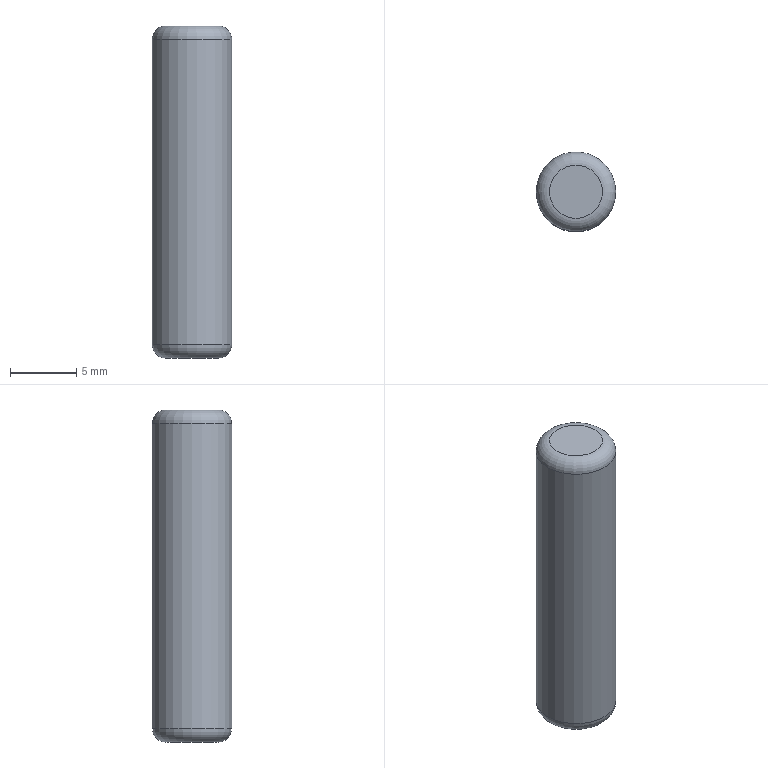Part | STEP file | 1 solid | 5 faces | box 6 x 6 x 25 mm | volume 699.37 mm3 | plane 2 | torus 2 | cylinder 1 | commonest cylinder face diameters 6 x1
STEP:
#1=CARTESIAN_POINT('',(0.,0.,0.));
#2=DIRECTION('',(0.,0.,1.));
#3=DIRECTION('',(1.,0.,0.));
#4=AXIS2_PLACEMENT_3D('',#1,#2,#3);
#5=CARTESIAN_POINT('',(1612.497,592.48,18.619));
#6=VERTEX_POINT('',#5);
#7=CARTESIAN_POINT('',(1610.497,592.48,18.619));
#8=DIRECTION('',(0.,0.,-1.));
#9=DIRECTION('',(1.,0.,0.));
#10=AXIS2_PLACEMENT_3D('',#7,#8,#9);
#11=CIRCLE('',#10,2.);
#12=CARTESIAN_POINT('',(1610.497,592.48,18.619));
#13=DIRECTION('',(0.,0.,-1.));
#14=DIRECTION('',(-1.,0.,0.));
#15=AXIS2_PLACEMENT_3D('',#12,#13,#14);
#16=PLANE('',#15);
#17=CARTESIAN_POINT('',(0.,0.));
#18=DIRECTION('',(-1.,0.));
#19=AXIS2_PLACEMENT_2D('',#17,#18);
#20=CIRCLE('',#19,2.);
#21=(GEOMETRIC_REPRESENTATION_CONTEXT(2)PARAMETRIC_REPRESENTATION_CONTEXT()REPRESENTATION_CONTEXT('',''));
#22=DEFINITIONAL_REPRESENTATION('',(#20),#21);
#23=PCURVE('',#16,#22);
#24=CARTESIAN_POINT('',(1610.497,592.48,19.619));
#25=DIRECTION('',(0.,0.,-1.));
#26=DIRECTION('',(-1.,0.,0.));
#27=AXIS2_PLACEMENT_3D('',#24,#25,#26);
#28=TOROIDAL_SURFACE('',#27,2.,1.);
#29=CARTESIAN_POINT('',(3.142,7.854));
#30=DIRECTION('',(1.,0.));
#31=VECTOR('',#30,1.);
#32=LINE('',#29,#31);
#33=(GEOMETRIC_REPRESENTATION_CONTEXT(2)PARAMETRIC_REPRESENTATION_CONTEXT()REPRESENTATION_CONTEXT('',''));
#34=DEFINITIONAL_REPRESENTATION('',(#32),#33);
#35=PCURVE('',#28,#34);
#36=SURFACE_CURVE('',#11,(#23,#35),.PCURVE_S1.);
#37=EDGE_CURVE('',#6,#6,#36,.T.);
#38=ORIENTED_EDGE('',*,*,#37,.T.);
#39=EDGE_LOOP('',(#38));
#40=FACE_BOUND('',#39,.T.);
#41=ADVANCED_FACE('',(#40),#16,.T.);
#42=CARTESIAN_POINT('',(1608.497,592.48,43.619));
#43=VERTEX_POINT('',#42);
#44=CARTESIAN_POINT('',(1610.497,592.48,43.619));
#45=DIRECTION('',(0.,0.,1.));
#46=DIRECTION('',(-1.,0.,0.));
#47=AXIS2_PLACEMENT_3D('',#44,#45,#46);
#48=CIRCLE('',#47,2.);
#49=CARTESIAN_POINT('',(1610.497,592.48,43.619));
#50=DIRECTION('',(0.,0.,1.));
#51=DIRECTION('',(1.,0.,0.));
#52=AXIS2_PLACEMENT_3D('',#49,#50,#51);
#53=PLANE('',#52);
#54=CARTESIAN_POINT('',(0.,0.));
#55=DIRECTION('',(-1.,0.));
#56=AXIS2_PLACEMENT_2D('',#54,#55);
#57=CIRCLE('',#56,2.);
#58=(GEOMETRIC_REPRESENTATION_CONTEXT(2)PARAMETRIC_REPRESENTATION_CONTEXT()REPRESENTATION_CONTEXT('',''));
#59=DEFINITIONAL_REPRESENTATION('',(#57),#58);
#60=PCURVE('',#53,#59);
#61=CARTESIAN_POINT('',(1610.497,592.48,42.619));
#62=DIRECTION('',(0.,0.,1.));
#63=DIRECTION('',(1.,0.,0.));
#64=AXIS2_PLACEMENT_3D('',#61,#62,#63);
#65=TOROIDAL_SURFACE('',#64,2.,1.);
#66=CARTESIAN_POINT('',(3.142,7.854));
#67=DIRECTION('',(1.,0.));
#68=VECTOR('',#67,1.);
#69=LINE('',#66,#68);
#70=(GEOMETRIC_REPRESENTATION_CONTEXT(2)PARAMETRIC_REPRESENTATION_CONTEXT()REPRESENTATION_CONTEXT('',''));
#71=DEFINITIONAL_REPRESENTATION('',(#69),#70);
#72=PCURVE('',#65,#71);
#73=SURFACE_CURVE('',#48,(#60,#72),.PCURVE_S1.);
#74=EDGE_CURVE('',#43,#43,#73,.T.);
#75=ORIENTED_EDGE('',*,*,#74,.T.);
#76=EDGE_LOOP('',(#75));
#77=FACE_BOUND('',#76,.T.);
#78=ADVANCED_FACE('',(#77),#53,.T.);
#79=CARTESIAN_POINT('',(1607.497,592.48,42.619));
#80=VERTEX_POINT('',#79);
#81=CARTESIAN_POINT('',(1610.497,592.48,42.619));
#82=DIRECTION('',(0.,0.,-1.));
#83=DIRECTION('',(-1.,0.,0.));
#84=AXIS2_PLACEMENT_3D('',#81,#82,#83);
#85=CIRCLE('',#84,3.);
#86=CARTESIAN_POINT('',(1610.497,592.48,33.619));
#87=DIRECTION('',(0.,0.,-1.));
#88=DIRECTION('',(-1.,0.,0.));
#89=AXIS2_PLACEMENT_3D('',#86,#87,#88);
#90=CYLINDRICAL_SURFACE('',#89,3.);
#91=CARTESIAN_POINT('',(0.,-9.));
#92=DIRECTION('',(1.,0.));
#93=VECTOR('',#92,1.);
#94=LINE('',#91,#93);
#95=(GEOMETRIC_REPRESENTATION_CONTEXT(2)PARAMETRIC_REPRESENTATION_CONTEXT()REPRESENTATION_CONTEXT('',''));
#96=DEFINITIONAL_REPRESENTATION('',(#94),#95);
#97=PCURVE('',#90,#96);
#98=CARTESIAN_POINT('',(9.425,6.283));
#99=DIRECTION('',(-1.,0.));
#100=VECTOR('',#99,1.);
#101=LINE('',#98,#100);
#102=(GEOMETRIC_REPRESENTATION_CONTEXT(2)PARAMETRIC_REPRESENTATION_CONTEXT()REPRESENTATION_CONTEXT('',''));
#103=DEFINITIONAL_REPRESENTATION('',(#101),#102);
#104=PCURVE('',#65,#103);
#105=SURFACE_CURVE('',#85,(#97,#104),.PCURVE_S1.);
#106=EDGE_CURVE('',#80,#80,#105,.T.);
#107=ORIENTED_EDGE('',*,*,#106,.T.);
#108=CARTESIAN_POINT('',(1607.497,592.48,19.619));
#109=VERTEX_POINT('',#108);
#110=CARTESIAN_POINT('',(1607.497,592.48,42.619));
#111=CARTESIAN_POINT('',(1607.497,592.48,19.619));
#112=B_SPLINE_CURVE_WITH_KNOTS('',1,(#110,#111),.UNSPECIFIED.,.F.,.F.,(2,2),(-9.,14.),.PIECEWISE_BEZIER_KNOTS.);
#113=CARTESIAN_POINT('',(6.283,0.));
#114=DIRECTION('',(0.,1.));
#115=VECTOR('',#114,1.);
#116=LINE('',#113,#115);
#117=(GEOMETRIC_REPRESENTATION_CONTEXT(2)PARAMETRIC_REPRESENTATION_CONTEXT()REPRESENTATION_CONTEXT('',''));
#118=DEFINITIONAL_REPRESENTATION('',(#116),#117);
#119=PCURVE('',#90,#118);
#120=CARTESIAN_POINT('',(0.,0.));
#121=DIRECTION('',(0.,1.));
#122=VECTOR('',#121,1.);
#123=LINE('',#120,#122);
#124=(GEOMETRIC_REPRESENTATION_CONTEXT(2)PARAMETRIC_REPRESENTATION_CONTEXT()REPRESENTATION_CONTEXT('',''));
#125=DEFINITIONAL_REPRESENTATION('',(#123),#124);
#126=PCURVE('',#90,#125);
#127=SEAM_CURVE('',#112,(#119,#126),.PCURVE_S1.);
#128=EDGE_CURVE('',#80,#109,#127,.T.);
#129=ORIENTED_EDGE('',*,*,#128,.T.);
#130=CARTESIAN_POINT('',(1613.497,592.48,19.619));
#131=VERTEX_POINT('',#130);
#132=CARTESIAN_POINT('',(1610.497,592.48,19.619));
#133=DIRECTION('',(0.,0.,1.));
#134=DIRECTION('',(1.,0.,0.));
#135=AXIS2_PLACEMENT_3D('',#132,#133,#134);
#136=CIRCLE('',#135,3.);
#137=CARTESIAN_POINT('',(9.425,14.));
#138=DIRECTION('',(-1.,0.));
#139=VECTOR('',#138,1.);
#140=LINE('',#137,#139);
#141=(GEOMETRIC_REPRESENTATION_CONTEXT(2)PARAMETRIC_REPRESENTATION_CONTEXT()REPRESENTATION_CONTEXT('',''));
#142=DEFINITIONAL_REPRESENTATION('',(#140),#141);
#143=PCURVE('',#90,#142);
#144=CARTESIAN_POINT('',(9.425,6.283));
#145=DIRECTION('',(-1.,0.));
#146=VECTOR('',#145,1.);
#147=LINE('',#144,#146);
#148=(GEOMETRIC_REPRESENTATION_CONTEXT(2)PARAMETRIC_REPRESENTATION_CONTEXT()REPRESENTATION_CONTEXT('',''));
#149=DEFINITIONAL_REPRESENTATION('',(#147),#148);
#150=PCURVE('',#28,#149);
#151=SURFACE_CURVE('',#136,(#143,#150),.PCURVE_S1.);
#152=EDGE_CURVE('',#109,#131,#151,.T.);
#153=ORIENTED_EDGE('',*,*,#152,.T.);
#154=CARTESIAN_POINT('',(1610.497,592.48,19.619));
#155=DIRECTION('',(0.,0.,1.));
#156=DIRECTION('',(1.,0.,0.));
#157=AXIS2_PLACEMENT_3D('',#154,#155,#156);
#158=CIRCLE('',#157,3.);
#159=CARTESIAN_POINT('',(3.142,14.));
#160=DIRECTION('',(-1.,0.));
#161=VECTOR('',#160,1.);
#162=LINE('',#159,#161);
#163=(GEOMETRIC_REPRESENTATION_CONTEXT(2)PARAMETRIC_REPRESENTATION_CONTEXT()REPRESENTATION_CONTEXT('',''));
#164=DEFINITIONAL_REPRESENTATION('',(#162),#163);
#165=PCURVE('',#90,#164);
#166=CARTESIAN_POINT('',(9.425,6.283));
#167=DIRECTION('',(-1.,0.));
#168=VECTOR('',#167,1.);
#169=LINE('',#166,#168);
#170=(GEOMETRIC_REPRESENTATION_CONTEXT(2)PARAMETRIC_REPRESENTATION_CONTEXT()REPRESENTATION_CONTEXT('',''));
#171=DEFINITIONAL_REPRESENTATION('',(#169),#170);
#172=PCURVE('',#28,#171);
#173=SURFACE_CURVE('',#158,(#165,#172),.PCURVE_S1.);
#174=EDGE_CURVE('',#131,#109,#173,.T.);
#175=ORIENTED_EDGE('',*,*,#174,.T.);
#176=ORIENTED_EDGE('',*,*,#128,.F.);
#177=EDGE_LOOP('',(#107,#129,#153,#175,#176));
#178=FACE_BOUND('',#177,.T.);
#179=ADVANCED_FACE('',(#178),#90,.T.);
#180=ORIENTED_EDGE('',*,*,#74,.F.);
#181=CARTESIAN_POINT('',(1607.497,592.48,42.619));
#182=CARTESIAN_POINT('',(1607.497,592.48,42.886));
#183=CARTESIAN_POINT('',(1607.582,592.48,43.147));
#184=CARTESIAN_POINT('',(1607.745,592.48,43.371));
#185=CARTESIAN_POINT('',(1607.97,592.48,43.534));
#186=CARTESIAN_POINT('',(1608.23,592.48,43.619));
#187=CARTESIAN_POINT('',(1608.497,592.48,43.619));
#188=(BOUNDED_CURVE()B_SPLINE_CURVE(6,(#181,#182,#183,#184,#185,#186,#187),.UNSPECIFIED.,.F.,.F.)B_SPLINE_CURVE_WITH_KNOTS((7,7),(0.,1.571),.PIECEWISE_BEZIER_KNOTS.)CURVE()GEOMETRIC_REPRESENTATION_ITEM()RATIONAL_B_SPLINE_CURVE((1.031,1.01,0.9979,0.994,0.9979,1.01,1.031))REPRESENTATION_ITEM(''));
#189=CARTESIAN_POINT('',(3.142,6.283));
#190=DIRECTION('',(0.,1.));
#191=VECTOR('',#190,1.);
#192=LINE('',#189,#191);
#193=(GEOMETRIC_REPRESENTATION_CONTEXT(2)PARAMETRIC_REPRESENTATION_CONTEXT()REPRESENTATION_CONTEXT('',''));
#194=DEFINITIONAL_REPRESENTATION('',(#192),#193);
#195=PCURVE('',#65,#194);
#196=CARTESIAN_POINT('',(9.425,6.283));
#197=DIRECTION('',(0.,1.));
#198=VECTOR('',#197,1.);
#199=LINE('',#196,#198);
#200=(GEOMETRIC_REPRESENTATION_CONTEXT(2)PARAMETRIC_REPRESENTATION_CONTEXT()REPRESENTATION_CONTEXT('',''));
#201=DEFINITIONAL_REPRESENTATION('',(#199),#200);
#202=PCURVE('',#65,#201);
#203=SEAM_CURVE('',#188,(#195,#202),.PCURVE_S1.);
#204=EDGE_CURVE('',#80,#43,#203,.T.);
#205=ORIENTED_EDGE('',*,*,#204,.F.);
#206=ORIENTED_EDGE('',*,*,#106,.F.);
#207=ORIENTED_EDGE('',*,*,#204,.T.);
#208=EDGE_LOOP('',(#180,#205,#206,#207));
#209=FACE_BOUND('',#208,.T.);
#210=ADVANCED_FACE('',(#209),#65,.T.);
#211=ORIENTED_EDGE('',*,*,#37,.F.);
#212=CARTESIAN_POINT('',(1613.497,592.48,19.619));
#213=CARTESIAN_POINT('',(1613.497,592.48,19.352));
#214=CARTESIAN_POINT('',(1613.412,592.48,19.091));
#215=CARTESIAN_POINT('',(1613.249,592.48,18.867));
#216=CARTESIAN_POINT('',(1613.025,592.48,18.704));
#217=CARTESIAN_POINT('',(1612.765,592.48,18.619));
#218=CARTESIAN_POINT('',(1612.497,592.48,18.619));
#219=(BOUNDED_CURVE()B_SPLINE_CURVE(6,(#212,#213,#214,#215,#216,#217,#218),.UNSPECIFIED.,.F.,.F.)B_SPLINE_CURVE_WITH_KNOTS((7,7),(0.,1.571),.PIECEWISE_BEZIER_KNOTS.)CURVE()GEOMETRIC_REPRESENTATION_ITEM()RATIONAL_B_SPLINE_CURVE((1.031,1.01,0.9979,0.994,0.9979,1.01,1.031))REPRESENTATION_ITEM(''));
#220=CARTESIAN_POINT('',(3.142,6.283));
#221=DIRECTION('',(0.,1.));
#222=VECTOR('',#221,1.);
#223=LINE('',#220,#222);
#224=(GEOMETRIC_REPRESENTATION_CONTEXT(2)PARAMETRIC_REPRESENTATION_CONTEXT()REPRESENTATION_CONTEXT('',''));
#225=DEFINITIONAL_REPRESENTATION('',(#223),#224);
#226=PCURVE('',#28,#225);
#227=CARTESIAN_POINT('',(9.425,6.283));
#228=DIRECTION('',(0.,1.));
#229=VECTOR('',#228,1.);
#230=LINE('',#227,#229);
#231=(GEOMETRIC_REPRESENTATION_CONTEXT(2)PARAMETRIC_REPRESENTATION_CONTEXT()REPRESENTATION_CONTEXT('',''));
#232=DEFINITIONAL_REPRESENTATION('',(#230),#231);
#233=PCURVE('',#28,#232);
#234=SEAM_CURVE('',#219,(#226,#233),.PCURVE_S1.);
#235=EDGE_CURVE('',#131,#6,#234,.T.);
#236=ORIENTED_EDGE('',*,*,#235,.F.);
#237=ORIENTED_EDGE('',*,*,#152,.F.);
#238=ORIENTED_EDGE('',*,*,#174,.F.);
#239=ORIENTED_EDGE('',*,*,#235,.T.);
#240=EDGE_LOOP('',(#211,#236,#237,#238,#239));
#241=FACE_BOUND('',#240,.T.);
#242=ADVANCED_FACE('',(#241),#28,.T.);
#243=CLOSED_SHELL('',(#41,#78,#179,#210,#242));
#244=MANIFOLD_SOLID_BREP('',#243);
#245=(LENGTH_UNIT()NAMED_UNIT(*)SI_UNIT(.MILLI.,.METRE.));
#246=UNCERTAINTY_MEASURE_WITH_UNIT(LENGTH_MEASURE(0.00001),#245,'','');
#247=(NAMED_UNIT(*)PLANE_ANGLE_UNIT()SI_UNIT($,.RADIAN.));
#248=(NAMED_UNIT(*)SI_UNIT($,.STERADIAN.)SOLID_ANGLE_UNIT());
#249=(GEOMETRIC_REPRESENTATION_CONTEXT(3)GLOBAL_UNCERTAINTY_ASSIGNED_CONTEXT((#246))GLOBAL_UNIT_ASSIGNED_CONTEXT((#245,#247,#248))REPRESENTATION_CONTEXT('',''));
#250=ADVANCED_BREP_SHAPE_REPRESENTATION('',(#4,#244),#249);